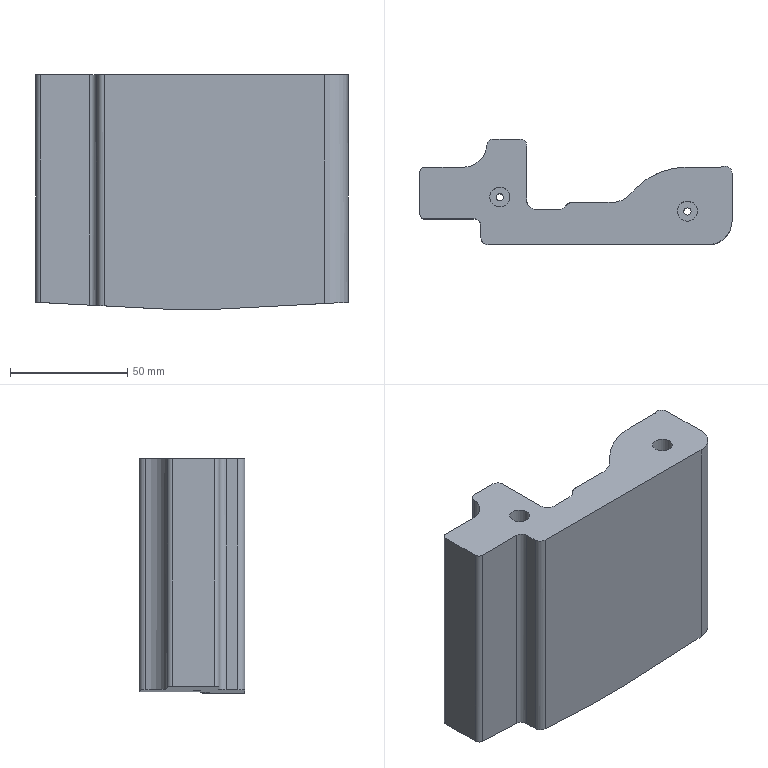Part | STEP file | lll_id234_x_t | 1 solid | 43 faces | box 133 x 45 x 100 mm | volume 339340 mm3 | cylinder 24 | plane 19 | commonest cylinder face diameters 6 x6 20 x3 3.1 x2 4 x2 8 x2 8.506 x2
STEP:
#1=CARTESIAN_POINT('',(1388.5,7.5,-7.5));
#2=VERTEX_POINT('',#1);
#3=CARTESIAN_POINT('',(1408.5,7.5,-7.5));
#4=VERTEX_POINT('',#3);
#5=CARTESIAN_POINT('',(1374.507,7.5,-7.5));
#6=DIRECTION('',(1.,0.,0.));
#7=VECTOR('',#6,1.);
#8=LINE('',#5,#7);
#9=EDGE_CURVE('',#2,#4,#8,.T.);
#10=ORIENTED_EDGE('',*,*,#9,.F.);
#11=CARTESIAN_POINT('',(1388.5,22.495,-7.5));
#12=VERTEX_POINT('',#11);
#13=CARTESIAN_POINT('',(1388.5,49.5,-7.5));
#14=DIRECTION('',(0.,-1.,0.));
#15=VECTOR('',#14,1.);
#16=LINE('',#13,#15);
#17=EDGE_CURVE('',#12,#2,#16,.T.);
#18=ORIENTED_EDGE('',*,*,#17,.F.);
#19=CARTESIAN_POINT('',(1391.,22.495,-7.5));
#20=VERTEX_POINT('',#19);
#21=CARTESIAN_POINT('',(1374.513,22.492,-7.5));
#22=DIRECTION('',(-1.,-0.0002273,0.));
#23=VECTOR('',#22,1.);
#24=LINE('',#21,#23);
#25=EDGE_CURVE('',#20,#12,#24,.T.);
#26=ORIENTED_EDGE('',*,*,#25,.F.);
#27=CARTESIAN_POINT('',(1394.112,23.983,-7.5));
#28=VERTEX_POINT('',#27);
#29=CARTESIAN_POINT('',(1390.999,26.495,-7.5));
#30=DIRECTION('',(0.,0.,-1.));
#31=DIRECTION('',(1.,0.,0.));
#32=AXIS2_PLACEMENT_3D('',#29,#30,#31);
#33=CIRCLE('',#32,4.);
#34=EDGE_CURVE('',#28,#20,#33,.T.);
#35=ORIENTED_EDGE('',*,*,#34,.F.);
#36=CARTESIAN_POINT('',(1394.775,24.627,-7.5));
#37=VERTEX_POINT('',#36);
#38=CARTESIAN_POINT('',(1397.092,21.579,-7.5));
#39=DIRECTION('',(0.,0.,1.));
#40=DIRECTION('',(1.,0.,0.));
#41=AXIS2_PLACEMENT_3D('',#38,#39,#40);
#42=CIRCLE('',#41,3.829);
#43=EDGE_CURVE('',#37,#28,#42,.T.);
#44=ORIENTED_EDGE('',*,*,#43,.F.);
#45=CARTESIAN_POINT('',(1395.716,25.182,-7.5));
#46=VERTEX_POINT('',#45);
#47=CARTESIAN_POINT('',(1397.363,21.312,-7.5));
#48=DIRECTION('',(0.,0.,1.));
#49=DIRECTION('',(1.,0.,0.));
#50=AXIS2_PLACEMENT_3D('',#47,#48,#49);
#51=CIRCLE('',#50,4.206);
#52=EDGE_CURVE('',#46,#37,#51,.T.);
#53=ORIENTED_EDGE('',*,*,#52,.F.);
#54=CARTESIAN_POINT('',(1396.385,25.384,-7.5));
#55=VERTEX_POINT('',#54);
#56=CARTESIAN_POINT('',(1397.014,22.085,-7.5));
#57=DIRECTION('',(0.,0.,1.));
#58=DIRECTION('',(1.,0.,0.));
#59=AXIS2_PLACEMENT_3D('',#56,#57,#58);
#60=CIRCLE('',#59,3.358);
#61=EDGE_CURVE('',#55,#46,#60,.T.);
#62=ORIENTED_EDGE('',*,*,#61,.F.);
#63=CARTESIAN_POINT('',(1396.692,25.434,-7.5));
#64=VERTEX_POINT('',#63);
#65=CARTESIAN_POINT('',(1397.334,20.531,-7.5));
#66=DIRECTION('',(0.,0.,-1.));
#67=DIRECTION('',(1.,0.,0.));
#68=AXIS2_PLACEMENT_3D('',#65,#66,#67);
#69=CIRCLE('',#68,4.944);
#70=EDGE_CURVE('',#55,#64,#69,.T.);
#71=ORIENTED_EDGE('',*,*,#70,.T.);
#72=CARTESIAN_POINT('',(1397.002,25.469,-7.5));
#73=VERTEX_POINT('',#72);
#74=CARTESIAN_POINT('',(1397.824,16.86,-7.5));
#75=DIRECTION('',(0.,0.,1.));
#76=DIRECTION('',(1.,0.,0.));
#77=AXIS2_PLACEMENT_3D('',#74,#75,#76);
#78=CIRCLE('',#77,8.648);
#79=EDGE_CURVE('',#73,#64,#78,.T.);
#80=ORIENTED_EDGE('',*,*,#79,.F.);
#81=CARTESIAN_POINT('',(1397.315,25.497,-7.5));
#82=VERTEX_POINT('',#81);
#83=CARTESIAN_POINT('',(1398.554,9.871,-7.5));
#84=DIRECTION('',(0.,0.,1.));
#85=DIRECTION('',(1.,0.,0.));
#86=AXIS2_PLACEMENT_3D('',#83,#84,#85);
#87=CIRCLE('',#86,15.675);
#88=EDGE_CURVE('',#82,#73,#87,.T.);
#89=ORIENTED_EDGE('',*,*,#88,.F.);
#90=CARTESIAN_POINT('',(1399.134,25.498,-7.5));
#91=VERTEX_POINT('',#90);
#92=CARTESIAN_POINT('',(1374.518,25.486,-7.5));
#93=DIRECTION('',(1.,0.0004734,0.));
#94=VECTOR('',#93,1.);
#95=LINE('',#92,#94);
#96=EDGE_CURVE('',#82,#91,#95,.T.);
#97=ORIENTED_EDGE('',*,*,#96,.T.);
#98=CARTESIAN_POINT('',(1408.5,25.502,-7.5));
#99=VERTEX_POINT('',#98);
#100=CARTESIAN_POINT('',(1374.517,25.488,-7.5));
#101=DIRECTION('',(1.,0.0004015,0.));
#102=VECTOR('',#101,1.);
#103=LINE('',#100,#102);
#104=EDGE_CURVE('',#91,#99,#103,.T.);
#105=ORIENTED_EDGE('',*,*,#104,.T.);
#106=CARTESIAN_POINT('',(1408.5,52.5,-7.5));
#107=DIRECTION('',(0.,1.,0.));
#108=VECTOR('',#107,1.);
#109=LINE('',#106,#108);
#110=EDGE_CURVE('',#4,#99,#109,.T.);
#111=ORIENTED_EDGE('',*,*,#110,.F.);
#112=EDGE_LOOP('',(#10,#18,#26,#35,#44,#53,#62,#71,#80,#89,#97,#105,#111));
#113=FACE_OUTER_BOUND('',#112,.T.);
#114=CARTESIAN_POINT('',(1374.507,49.5,-7.5));
#115=DIRECTION('',(0.,0.,1.));
#116=DIRECTION('',(-1.,0.,0.));
#117=AXIS2_PLACEMENT_3D('',#114,#115,#116);
#118=PLANE('',#117);
#119=ADVANCED_FACE('',(#113),#118,.F.);
#120=CARTESIAN_POINT('',(1370.253,27.75,92.5));
#121=VERTEX_POINT('',#120);
#122=CARTESIAN_POINT('',(1366.,27.75,92.5));
#123=DIRECTION('',(0.,0.,-1.));
#124=DIRECTION('',(1.,0.,0.));
#125=AXIS2_PLACEMENT_3D('',#122,#123,#124);
#126=CIRCLE('',#125,4.253);
#127=EDGE_CURVE('',#121,#121,#126,.T.);
#128=ORIENTED_EDGE('',*,*,#127,.T.);
#129=EDGE_LOOP('',(#128));
#130=FACE_BOUND('',#129,.T.);
#131=CARTESIAN_POINT('',(1450.253,21.75,92.5));
#132=VERTEX_POINT('',#131);
#133=CARTESIAN_POINT('',(1446.,21.75,92.5));
#134=DIRECTION('',(0.,0.,-1.));
#135=DIRECTION('',(1.,0.,0.));
#136=AXIS2_PLACEMENT_3D('',#133,#134,#135);
#137=CIRCLE('',#136,4.253);
#138=EDGE_CURVE('',#132,#132,#137,.T.);
#139=ORIENTED_EDGE('',*,*,#138,.T.);
#140=EDGE_LOOP('',(#139));
#141=FACE_BOUND('',#140,.T.);
#142=CARTESIAN_POINT('',(1394.775,24.627,92.5));
#143=VERTEX_POINT('',#142);
#144=CARTESIAN_POINT('',(1395.716,25.182,92.5));
#145=VERTEX_POINT('',#144);
#146=CARTESIAN_POINT('',(1397.363,21.312,92.5));
#147=DIRECTION('',(0.,0.,-1.));
#148=DIRECTION('',(1.,0.,0.));
#149=AXIS2_PLACEMENT_3D('',#146,#147,#148);
#150=CIRCLE('',#149,4.206);
#151=EDGE_CURVE('',#143,#145,#150,.T.);
#152=ORIENTED_EDGE('',*,*,#151,.F.);
#153=CARTESIAN_POINT('',(1394.112,23.983,92.5));
#154=VERTEX_POINT('',#153);
#155=CARTESIAN_POINT('',(1397.092,21.579,92.5));
#156=DIRECTION('',(0.,0.,1.));
#157=DIRECTION('',(1.,0.,0.));
#158=AXIS2_PLACEMENT_3D('',#155,#156,#157);
#159=CIRCLE('',#158,3.829);
#160=EDGE_CURVE('',#143,#154,#159,.T.);
#161=ORIENTED_EDGE('',*,*,#160,.T.);
#162=CARTESIAN_POINT('',(1391.,22.495,92.5));
#163=VERTEX_POINT('',#162);
#164=CARTESIAN_POINT('',(1390.999,26.495,92.5));
#165=DIRECTION('',(0.,0.,-1.));
#166=DIRECTION('',(1.,0.,0.));
#167=AXIS2_PLACEMENT_3D('',#164,#165,#166);
#168=CIRCLE('',#167,4.);
#169=EDGE_CURVE('',#154,#163,#168,.T.);
#170=ORIENTED_EDGE('',*,*,#169,.T.);
#171=CARTESIAN_POINT('',(1381.51,22.493,92.5));
#172=VERTEX_POINT('',#171);
#173=CARTESIAN_POINT('',(1374.513,22.492,92.5));
#174=DIRECTION('',(-1.,-0.0002273,0.));
#175=VECTOR('',#174,1.);
#176=LINE('',#173,#175);
#177=EDGE_CURVE('',#163,#172,#176,.T.);
#178=ORIENTED_EDGE('',*,*,#177,.T.);
#179=CARTESIAN_POINT('',(1377.509,26.493,92.5));
#180=VERTEX_POINT('',#179);
#181=CARTESIAN_POINT('',(1381.509,26.493,92.5));
#182=DIRECTION('',(0.,0.,1.));
#183=DIRECTION('',(1.,0.,0.));
#184=AXIS2_PLACEMENT_3D('',#181,#182,#183);
#185=CIRCLE('',#184,4.);
#186=EDGE_CURVE('',#180,#172,#185,.T.);
#187=ORIENTED_EDGE('',*,*,#186,.F.);
#188=CARTESIAN_POINT('',(1377.507,49.5,92.5));
#189=VERTEX_POINT('',#188);
#190=CARTESIAN_POINT('',(1377.507,49.5,92.5));
#191=DIRECTION('',(0.00008306,-1.,0.));
#192=VECTOR('',#191,1.);
#193=LINE('',#190,#192);
#194=EDGE_CURVE('',#189,#180,#193,.T.);
#195=ORIENTED_EDGE('',*,*,#194,.F.);
#196=CARTESIAN_POINT('',(1374.507,52.5,92.5));
#197=VERTEX_POINT('',#196);
#198=CARTESIAN_POINT('',(1374.507,49.5,92.5));
#199=DIRECTION('',(0.,0.,1.));
#200=DIRECTION('',(1.,0.,0.));
#201=AXIS2_PLACEMENT_3D('',#198,#199,#200);
#202=CIRCLE('',#201,3.);
#203=EDGE_CURVE('',#189,#197,#202,.T.);
#204=ORIENTED_EDGE('',*,*,#203,.T.);
#205=CARTESIAN_POINT('',(1363.461,52.5,92.5));
#206=VERTEX_POINT('',#205);
#207=CARTESIAN_POINT('',(1374.507,52.5,92.5));
#208=DIRECTION('',(-1.,0.,0.));
#209=VECTOR('',#208,1.);
#210=LINE('',#207,#209);
#211=EDGE_CURVE('',#197,#206,#210,.T.);
#212=ORIENTED_EDGE('',*,*,#211,.T.);
#213=CARTESIAN_POINT('',(1360.47,49.731,92.5));
#214=VERTEX_POINT('',#213);
#215=CARTESIAN_POINT('',(1363.461,49.5,92.5));
#216=DIRECTION('',(0.,0.,-1.));
#217=DIRECTION('',(1.,0.,0.));
#218=AXIS2_PLACEMENT_3D('',#215,#216,#217);
#219=CIRCLE('',#218,3.);
#220=EDGE_CURVE('',#214,#206,#219,.T.);
#221=ORIENTED_EDGE('',*,*,#220,.F.);
#222=CARTESIAN_POINT('',(1350.5,40.5,92.5));
#223=VERTEX_POINT('',#222);
#224=CARTESIAN_POINT('',(1350.5,50.5,92.5));
#225=DIRECTION('',(0.,0.,1.));
#226=DIRECTION('',(1.,0.,0.));
#227=AXIS2_PLACEMENT_3D('',#224,#225,#226);
#228=CIRCLE('',#227,10.);
#229=EDGE_CURVE('',#223,#214,#228,.T.);
#230=ORIENTED_EDGE('',*,*,#229,.F.);
#231=CARTESIAN_POINT('',(1334.,40.5,92.5));
#232=VERTEX_POINT('',#231);
#233=CARTESIAN_POINT('',(1374.507,40.5,92.5));
#234=DIRECTION('',(1.,0.,0.));
#235=VECTOR('',#234,1.);
#236=LINE('',#233,#235);
#237=EDGE_CURVE('',#232,#223,#236,.T.);
#238=ORIENTED_EDGE('',*,*,#237,.F.);
#239=CARTESIAN_POINT('',(1332.,38.5,92.5));
#240=VERTEX_POINT('',#239);
#241=CARTESIAN_POINT('',(1334.,38.5,92.5));
#242=DIRECTION('',(0.,0.,1.));
#243=DIRECTION('',(1.,0.,0.));
#244=AXIS2_PLACEMENT_3D('',#241,#242,#243);
#245=CIRCLE('',#244,2.);
#246=EDGE_CURVE('',#232,#240,#245,.T.);
#247=ORIENTED_EDGE('',*,*,#246,.T.);
#248=CARTESIAN_POINT('',(1332.,20.5,92.5));
#249=VERTEX_POINT('',#248);
#250=CARTESIAN_POINT('',(1332.,49.5,92.5));
#251=DIRECTION('',(0.,1.,0.));
#252=VECTOR('',#251,1.);
#253=LINE('',#250,#252);
#254=EDGE_CURVE('',#249,#240,#253,.T.);
#255=ORIENTED_EDGE('',*,*,#254,.F.);
#256=CARTESIAN_POINT('',(1334.,18.5,92.5));
#257=VERTEX_POINT('',#256);
#258=CARTESIAN_POINT('',(1334.,20.5,92.5));
#259=DIRECTION('',(0.,0.,1.));
#260=DIRECTION('',(1.,0.,0.));
#261=AXIS2_PLACEMENT_3D('',#258,#259,#260);
#262=CIRCLE('',#261,2.);
#263=EDGE_CURVE('',#249,#257,#262,.T.);
#264=ORIENTED_EDGE('',*,*,#263,.T.);
#265=CARTESIAN_POINT('',(1355.,18.5,92.5));
#266=VERTEX_POINT('',#265);
#267=CARTESIAN_POINT('',(1374.507,18.5,92.5));
#268=DIRECTION('',(1.,0.,0.));
#269=VECTOR('',#268,1.);
#270=LINE('',#267,#269);
#271=EDGE_CURVE('',#257,#266,#270,.T.);
#272=ORIENTED_EDGE('',*,*,#271,.T.);
#273=CARTESIAN_POINT('',(1358.,15.5,92.5));
#274=VERTEX_POINT('',#273);
#275=CARTESIAN_POINT('',(1355.,15.5,92.5));
#276=DIRECTION('',(0.,0.,1.));
#277=DIRECTION('',(1.,0.,0.));
#278=AXIS2_PLACEMENT_3D('',#275,#276,#277);
#279=CIRCLE('',#278,3.);
#280=EDGE_CURVE('',#274,#266,#279,.T.);
#281=ORIENTED_EDGE('',*,*,#280,.F.);
#282=CARTESIAN_POINT('',(1358.,10.5,92.5));
#283=VERTEX_POINT('',#282);
#284=CARTESIAN_POINT('',(1358.,49.5,92.5));
#285=DIRECTION('',(0.,1.,0.));
#286=VECTOR('',#285,1.);
#287=LINE('',#284,#286);
#288=EDGE_CURVE('',#283,#274,#287,.T.);
#289=ORIENTED_EDGE('',*,*,#288,.F.);
#290=CARTESIAN_POINT('',(1361.,7.5,92.5));
#291=VERTEX_POINT('',#290);
#292=CARTESIAN_POINT('',(1361.,10.5,92.5));
#293=DIRECTION('',(0.,0.,-1.));
#294=DIRECTION('',(1.,0.,0.));
#295=AXIS2_PLACEMENT_3D('',#292,#293,#294);
#296=CIRCLE('',#295,3.);
#297=EDGE_CURVE('',#291,#283,#296,.T.);
#298=ORIENTED_EDGE('',*,*,#297,.F.);
#299=CARTESIAN_POINT('',(1455.,7.5,92.5));
#300=VERTEX_POINT('',#299);
#301=CARTESIAN_POINT('',(1374.507,7.5,92.5));
#302=DIRECTION('',(1.,0.,0.));
#303=VECTOR('',#302,1.);
#304=LINE('',#301,#303);
#305=EDGE_CURVE('',#291,#300,#304,.T.);
#306=ORIENTED_EDGE('',*,*,#305,.T.);
#307=CARTESIAN_POINT('',(1465.,17.5,92.5));
#308=VERTEX_POINT('',#307);
#309=CARTESIAN_POINT('',(1455.,17.5,92.5));
#310=DIRECTION('',(0.,0.,-1.));
#311=DIRECTION('',(1.,0.,0.));
#312=AXIS2_PLACEMENT_3D('',#309,#310,#311);
#313=CIRCLE('',#312,10.);
#314=EDGE_CURVE('',#308,#300,#313,.T.);
#315=ORIENTED_EDGE('',*,*,#314,.F.);
#316=CARTESIAN_POINT('',(1465.,38.,92.5));
#317=VERTEX_POINT('',#316);
#318=CARTESIAN_POINT('',(1465.,49.5,92.5));
#319=DIRECTION('',(0.,1.,0.));
#320=VECTOR('',#319,1.);
#321=LINE('',#318,#320);
#322=EDGE_CURVE('',#308,#317,#321,.T.);
#323=ORIENTED_EDGE('',*,*,#322,.T.);
#324=CARTESIAN_POINT('',(1460.801,40.75,92.5));
#325=VERTEX_POINT('',#324);
#326=CARTESIAN_POINT('',(1462.,38.,92.5));
#327=DIRECTION('',(0.,0.,1.));
#328=DIRECTION('',(1.,0.,0.));
#329=AXIS2_PLACEMENT_3D('',#326,#327,#328);
#330=CIRCLE('',#329,3.);
#331=EDGE_CURVE('',#317,#325,#330,.T.);
#332=ORIENTED_EDGE('',*,*,#331,.T.);
#333=CARTESIAN_POINT('',(1459.602,40.5,92.5));
#334=VERTEX_POINT('',#333);
#335=CARTESIAN_POINT('',(1459.602,43.5,92.5));
#336=DIRECTION('',(0.,0.,-1.));
#337=DIRECTION('',(1.,0.,0.));
#338=AXIS2_PLACEMENT_3D('',#335,#336,#337);
#339=CIRCLE('',#338,3.);
#340=EDGE_CURVE('',#325,#334,#339,.T.);
#341=ORIENTED_EDGE('',*,*,#340,.T.);
#342=CARTESIAN_POINT('',(1445.426,40.5,92.5));
#343=VERTEX_POINT('',#342);
#344=CARTESIAN_POINT('',(1374.507,40.5,92.5));
#345=DIRECTION('',(1.,0.,0.));
#346=VECTOR('',#345,1.);
#347=LINE('',#344,#346);
#348=EDGE_CURVE('',#343,#334,#347,.T.);
#349=ORIENTED_EDGE('',*,*,#348,.F.);
#350=CARTESIAN_POINT('',(1424.213,31.713,92.5));
#351=VERTEX_POINT('',#350);
#352=CARTESIAN_POINT('',(1445.426,10.502,92.5));
#353=DIRECTION('',(0.,0.,-1.));
#354=DIRECTION('',(1.,0.,0.));
#355=AXIS2_PLACEMENT_3D('',#352,#353,#354);
#356=CIRCLE('',#355,29.998);
#357=EDGE_CURVE('',#351,#343,#356,.T.);
#358=ORIENTED_EDGE('',*,*,#357,.F.);
#359=CARTESIAN_POINT('',(1420.933,28.433,92.5));
#360=VERTEX_POINT('',#359);
#361=CARTESIAN_POINT('',(1408.253,15.754,92.5));
#362=DIRECTION('',(-0.7071,-0.7071,0.));
#363=VECTOR('',#362,1.);
#364=LINE('',#361,#363);
#365=EDGE_CURVE('',#351,#360,#364,.T.);
#366=ORIENTED_EDGE('',*,*,#365,.T.);
#367=CARTESIAN_POINT('',(1413.865,25.504,92.5));
#368=VERTEX_POINT('',#367);
#369=CARTESIAN_POINT('',(1413.861,35.504,92.5));
#370=DIRECTION('',(0.,0.,-1.));
#371=DIRECTION('',(1.,0.,0.));
#372=AXIS2_PLACEMENT_3D('',#369,#370,#371);
#373=CIRCLE('',#372,10.);
#374=EDGE_CURVE('',#360,#368,#373,.T.);
#375=ORIENTED_EDGE('',*,*,#374,.T.);
#376=CARTESIAN_POINT('',(1399.134,25.498,92.5));
#377=VERTEX_POINT('',#376);
#378=CARTESIAN_POINT('',(1374.517,25.488,92.5));
#379=DIRECTION('',(-1.,-0.0004015,0.));
#380=VECTOR('',#379,1.);
#381=LINE('',#378,#380);
#382=EDGE_CURVE('',#368,#377,#381,.T.);
#383=ORIENTED_EDGE('',*,*,#382,.T.);
#384=CARTESIAN_POINT('',(1397.315,25.497,92.5));
#385=VERTEX_POINT('',#384);
#386=CARTESIAN_POINT('',(1374.518,25.486,92.5));
#387=DIRECTION('',(1.,0.0004734,0.));
#388=VECTOR('',#387,1.);
#389=LINE('',#386,#388);
#390=EDGE_CURVE('',#385,#377,#389,.T.);
#391=ORIENTED_EDGE('',*,*,#390,.F.);
#392=CARTESIAN_POINT('',(1397.002,25.469,92.5));
#393=VERTEX_POINT('',#392);
#394=CARTESIAN_POINT('',(1398.554,9.871,92.5));
#395=DIRECTION('',(0.,0.,1.));
#396=DIRECTION('',(1.,0.,0.));
#397=AXIS2_PLACEMENT_3D('',#394,#395,#396);
#398=CIRCLE('',#397,15.675);
#399=EDGE_CURVE('',#385,#393,#398,.T.);
#400=ORIENTED_EDGE('',*,*,#399,.T.);
#401=CARTESIAN_POINT('',(1396.692,25.434,92.5));
#402=VERTEX_POINT('',#401);
#403=CARTESIAN_POINT('',(1397.824,16.86,92.5));
#404=DIRECTION('',(0.,0.,-1.));
#405=DIRECTION('',(1.,0.,0.));
#406=AXIS2_PLACEMENT_3D('',#403,#404,#405);
#407=CIRCLE('',#406,8.648);
#408=EDGE_CURVE('',#402,#393,#407,.T.);
#409=ORIENTED_EDGE('',*,*,#408,.F.);
#410=CARTESIAN_POINT('',(1396.385,25.384,92.5));
#411=VERTEX_POINT('',#410);
#412=CARTESIAN_POINT('',(1397.334,20.531,92.5));
#413=DIRECTION('',(0.,0.,1.));
#414=DIRECTION('',(1.,0.,0.));
#415=AXIS2_PLACEMENT_3D('',#412,#413,#414);
#416=CIRCLE('',#415,4.944);
#417=EDGE_CURVE('',#402,#411,#416,.T.);
#418=ORIENTED_EDGE('',*,*,#417,.T.);
#419=CARTESIAN_POINT('',(1397.014,22.085,92.5));
#420=DIRECTION('',(0.,0.,-1.));
#421=DIRECTION('',(1.,0.,0.));
#422=AXIS2_PLACEMENT_3D('',#419,#420,#421);
#423=CIRCLE('',#422,3.358);
#424=EDGE_CURVE('',#145,#411,#423,.T.);
#425=ORIENTED_EDGE('',*,*,#424,.F.);
#426=EDGE_LOOP('',(#152,#161,#170,#178,#187,#195,#204,#212,#221,#230,#238,#247,#255,#264,#272,#281,#289,#298,#306,#315,#323,#332,#341,#349,#358,#366,#375,#383,#391,#400,#409,#418,#425));
#427=FACE_BOUND('',#426,.T.);
#428=CARTESIAN_POINT('',(1374.507,49.5,92.5));
#429=DIRECTION('',(0.,0.,1.));
#430=DIRECTION('',(-1.,0.,0.));
#431=AXIS2_PLACEMENT_3D('',#428,#429,#430);
#432=PLANE('',#431);
#433=ADVANCED_FACE('',(#130,#141,#427),#432,.T.);
#434=CARTESIAN_POINT('',(1444.45,21.75,-5.591));
#435=VERTEX_POINT('',#434);
#436=CARTESIAN_POINT('',(1446.,21.75,-5.509));
#437=DIRECTION('',(-0.05302,0.,0.9986));
#438=DIRECTION('',(-0.9986,0.,-0.05302));
#439=AXIS2_PLACEMENT_3D('',#436,#437,#438);
#440=ELLIPSE('',#439,1.552,1.55);
#441=EDGE_CURVE('',#435,#435,#440,.T.);
#442=ORIENTED_EDGE('',*,*,#441,.T.);
#443=EDGE_LOOP('',(#442));
#444=FACE_BOUND('',#443,.T.);
#445=CARTESIAN_POINT('',(1455.,7.5,-5.031));
#446=VERTEX_POINT('',#445);
#447=CARTESIAN_POINT('',(1465.,17.5,-4.5));
#448=VERTEX_POINT('',#447);
#449=CARTESIAN_POINT('',(1455.,17.5,-5.031));
#450=DIRECTION('',(-0.05302,0.,0.9986));
#451=DIRECTION('',(0.9986,0.,0.05302));
#452=AXIS2_PLACEMENT_3D('',#449,#450,#451);
#453=ELLIPSE('',#452,10.014,10.);
#454=EDGE_CURVE('',#446,#448,#453,.T.);
#455=ORIENTED_EDGE('',*,*,#454,.F.);
#456=CARTESIAN_POINT('',(1408.5,7.5,-7.5));
#457=DIRECTION('',(0.9986,0.,0.05302));
#458=VECTOR('',#457,1.);
#459=LINE('',#456,#458);
#460=EDGE_CURVE('',#4,#446,#459,.T.);
#461=ORIENTED_EDGE('',*,*,#460,.F.);
#462=ORIENTED_EDGE('',*,*,#110,.T.);
#463=CARTESIAN_POINT('',(1413.865,25.504,-7.215));
#464=VERTEX_POINT('',#463);
#465=CARTESIAN_POINT('',(1408.511,25.502,-7.499));
#466=DIRECTION('',(0.9986,0.0004009,0.05302));
#467=VECTOR('',#466,1.);
#468=LINE('',#465,#467);
#469=EDGE_CURVE('',#99,#464,#468,.T.);
#470=ORIENTED_EDGE('',*,*,#469,.T.);
#471=CARTESIAN_POINT('',(1420.933,28.433,-6.84));
#472=VERTEX_POINT('',#471);
#473=CARTESIAN_POINT('',(1413.861,35.504,-7.215));
#474=DIRECTION('',(0.05302,0.,-0.9986));
#475=DIRECTION('',(0.9986,0.,0.05302));
#476=AXIS2_PLACEMENT_3D('',#473,#474,#475);
#477=ELLIPSE('',#476,10.014,10.);
#478=EDGE_CURVE('',#472,#464,#477,.T.);
#479=ORIENTED_EDGE('',*,*,#478,.F.);
#480=CARTESIAN_POINT('',(1424.213,31.713,-6.666));
#481=VERTEX_POINT('',#480);
#482=CARTESIAN_POINT('',(1426.724,34.224,-6.532));
#483=DIRECTION('',(0.7066,0.7066,0.03752));
#484=VECTOR('',#483,1.);
#485=LINE('',#482,#484);
#486=EDGE_CURVE('',#472,#481,#485,.T.);
#487=ORIENTED_EDGE('',*,*,#486,.T.);
#488=CARTESIAN_POINT('',(1445.426,40.5,-5.539));
#489=VERTEX_POINT('',#488);
#490=CARTESIAN_POINT('',(1445.426,10.502,-5.539));
#491=DIRECTION('',(-0.05302,0.,0.9986));
#492=DIRECTION('',(0.9986,0.,0.05302));
#493=AXIS2_PLACEMENT_3D('',#490,#491,#492);
#494=ELLIPSE('',#493,30.04,29.998);
#495=EDGE_CURVE('',#489,#481,#494,.T.);
#496=ORIENTED_EDGE('',*,*,#495,.F.);
#497=CARTESIAN_POINT('',(1459.602,40.5,-4.787));
#498=VERTEX_POINT('',#497);
#499=CARTESIAN_POINT('',(1408.5,40.5,-7.5));
#500=DIRECTION('',(0.9986,0.,0.05302));
#501=VECTOR('',#500,1.);
#502=LINE('',#499,#501);
#503=EDGE_CURVE('',#489,#498,#502,.T.);
#504=ORIENTED_EDGE('',*,*,#503,.T.);
#505=CARTESIAN_POINT('',(1460.801,40.75,-4.723));
#506=VERTEX_POINT('',#505);
#507=CARTESIAN_POINT('',(1459.602,43.5,-4.787));
#508=DIRECTION('',(-0.05302,0.,0.9986));
#509=DIRECTION('',(0.9986,0.,0.05302));
#510=AXIS2_PLACEMENT_3D('',#507,#508,#509);
#511=ELLIPSE('',#510,3.004,3.);
#512=EDGE_CURVE('',#498,#506,#511,.T.);
#513=ORIENTED_EDGE('',*,*,#512,.T.);
#514=CARTESIAN_POINT('',(1465.,38.,-4.5));
#515=VERTEX_POINT('',#514);
#516=CARTESIAN_POINT('',(1462.,38.,-4.659));
#517=DIRECTION('',(0.05302,0.,-0.9986));
#518=DIRECTION('',(0.9986,0.,0.05302));
#519=AXIS2_PLACEMENT_3D('',#516,#517,#518);
#520=ELLIPSE('',#519,3.004,3.);
#521=EDGE_CURVE('',#506,#515,#520,.T.);
#522=ORIENTED_EDGE('',*,*,#521,.T.);
#523=CARTESIAN_POINT('',(1465.,52.5,-4.5));
#524=DIRECTION('',(0.,-1.,0.));
#525=VECTOR('',#524,1.);
#526=LINE('',#523,#525);
#527=EDGE_CURVE('',#515,#448,#526,.T.);
#528=ORIENTED_EDGE('',*,*,#527,.T.);
#529=EDGE_LOOP('',(#455,#461,#462,#470,#479,#487,#496,#504,#513,#522,#528));
#530=FACE_BOUND('',#529,.T.);
#531=CARTESIAN_POINT('',(1408.5,52.5,-7.5));
#532=DIRECTION('',(0.05302,0.,-0.9986));
#533=DIRECTION('',(-0.9986,0.,-0.05302));
#534=AXIS2_PLACEMENT_3D('',#531,#532,#533);
#535=PLANE('',#534);
#536=ADVANCED_FACE('',(#444,#530),#535,.T.);
#537=CARTESIAN_POINT('',(1367.55,27.75,-6.388));
#538=VERTEX_POINT('',#537);
#539=CARTESIAN_POINT('',(1366.,27.75,-6.305));
#540=DIRECTION('',(-0.05302,0.,-0.9986));
#541=DIRECTION('',(0.9986,0.,-0.05302));
#542=AXIS2_PLACEMENT_3D('',#539,#540,#541);
#543=ELLIPSE('',#542,1.552,1.55);
#544=EDGE_CURVE('',#538,#538,#543,.T.);
#545=ORIENTED_EDGE('',*,*,#544,.F.);
#546=EDGE_LOOP('',(#545));
#547=FACE_BOUND('',#546,.T.);
#548=CARTESIAN_POINT('',(1381.51,22.493,-7.129));
#549=VERTEX_POINT('',#548);
#550=CARTESIAN_POINT('',(1388.507,22.495,-7.5));
#551=DIRECTION('',(-0.9986,-0.000227,0.05302));
#552=VECTOR('',#551,1.);
#553=LINE('',#550,#552);
#554=EDGE_CURVE('',#12,#549,#553,.T.);
#555=ORIENTED_EDGE('',*,*,#554,.F.);
#556=ORIENTED_EDGE('',*,*,#17,.T.);
#557=CARTESIAN_POINT('',(1361.,7.5,-6.04));
#558=VERTEX_POINT('',#557);
#559=CARTESIAN_POINT('',(1388.5,7.5,-7.5));
#560=DIRECTION('',(-0.9986,0.,0.05302));
#561=VECTOR('',#560,1.);
#562=LINE('',#559,#561);
#563=EDGE_CURVE('',#2,#558,#562,.T.);
#564=ORIENTED_EDGE('',*,*,#563,.T.);
#565=CARTESIAN_POINT('',(1358.,10.5,-5.881));
#566=VERTEX_POINT('',#565);
#567=CARTESIAN_POINT('',(1361.,10.5,-6.04));
#568=DIRECTION('',(0.05302,0.,0.9986));
#569=DIRECTION('',(-0.9986,0.,0.05302));
#570=AXIS2_PLACEMENT_3D('',#567,#568,#569);
#571=ELLIPSE('',#570,3.004,3.);
#572=EDGE_CURVE('',#566,#558,#571,.T.);
#573=ORIENTED_EDGE('',*,*,#572,.F.);
#574=CARTESIAN_POINT('',(1358.,15.5,-5.881));
#575=VERTEX_POINT('',#574);
#576=CARTESIAN_POINT('',(1358.,52.5,-5.881));
#577=DIRECTION('',(0.,-1.,0.));
#578=VECTOR('',#577,1.);
#579=LINE('',#576,#578);
#580=EDGE_CURVE('',#575,#566,#579,.T.);
#581=ORIENTED_EDGE('',*,*,#580,.F.);
#582=CARTESIAN_POINT('',(1355.,18.5,-5.721));
#583=VERTEX_POINT('',#582);
#584=CARTESIAN_POINT('',(1355.,15.5,-5.721));
#585=DIRECTION('',(-0.05302,0.,-0.9986));
#586=DIRECTION('',(-0.9986,0.,0.05302));
#587=AXIS2_PLACEMENT_3D('',#584,#585,#586);
#588=ELLIPSE('',#587,3.004,3.);
#589=EDGE_CURVE('',#583,#575,#588,.T.);
#590=ORIENTED_EDGE('',*,*,#589,.F.);
#591=CARTESIAN_POINT('',(1334.,18.5,-4.606));
#592=VERTEX_POINT('',#591);
#593=CARTESIAN_POINT('',(1388.5,18.5,-7.5));
#594=DIRECTION('',(0.9986,0.,-0.05302));
#595=VECTOR('',#594,1.);
#596=LINE('',#593,#595);
#597=EDGE_CURVE('',#592,#583,#596,.T.);
#598=ORIENTED_EDGE('',*,*,#597,.F.);
#599=CARTESIAN_POINT('',(1332.,20.5,-4.5));
#600=VERTEX_POINT('',#599);
#601=CARTESIAN_POINT('',(1334.,20.5,-4.606));
#602=DIRECTION('',(0.05302,0.,0.9986));
#603=DIRECTION('',(-0.9986,0.,0.05302));
#604=AXIS2_PLACEMENT_3D('',#601,#602,#603);
#605=ELLIPSE('',#604,2.003,2.);
#606=EDGE_CURVE('',#600,#592,#605,.T.);
#607=ORIENTED_EDGE('',*,*,#606,.F.);
#608=CARTESIAN_POINT('',(1332.,38.5,-4.5));
#609=VERTEX_POINT('',#608);
#610=CARTESIAN_POINT('',(1332.,52.5,-4.5));
#611=DIRECTION('',(0.,1.,0.));
#612=VECTOR('',#611,1.);
#613=LINE('',#610,#612);
#614=EDGE_CURVE('',#600,#609,#613,.T.);
#615=ORIENTED_EDGE('',*,*,#614,.T.);
#616=CARTESIAN_POINT('',(1334.,40.5,-4.606));
#617=VERTEX_POINT('',#616);
#618=CARTESIAN_POINT('',(1334.,38.5,-4.606));
#619=DIRECTION('',(0.05302,0.,0.9986));
#620=DIRECTION('',(-0.9986,0.,0.05302));
#621=AXIS2_PLACEMENT_3D('',#618,#619,#620);
#622=ELLIPSE('',#621,2.003,2.);
#623=EDGE_CURVE('',#617,#609,#622,.T.);
#624=ORIENTED_EDGE('',*,*,#623,.F.);
#625=CARTESIAN_POINT('',(1350.5,40.5,-5.482));
#626=VERTEX_POINT('',#625);
#627=CARTESIAN_POINT('',(1388.5,40.5,-7.5));
#628=DIRECTION('',(-0.9986,0.,0.05302));
#629=VECTOR('',#628,1.);
#630=LINE('',#627,#629);
#631=EDGE_CURVE('',#626,#617,#630,.T.);
#632=ORIENTED_EDGE('',*,*,#631,.F.);
#633=CARTESIAN_POINT('',(1360.47,49.731,-6.012));
#634=VERTEX_POINT('',#633);
#635=CARTESIAN_POINT('',(1350.5,50.5,-5.482));
#636=DIRECTION('',(-0.05302,0.,-0.9986));
#637=DIRECTION('',(-0.9986,0.,0.05302));
#638=AXIS2_PLACEMENT_3D('',#635,#636,#637);
#639=ELLIPSE('',#638,10.014,10.);
#640=EDGE_CURVE('',#634,#626,#639,.T.);
#641=ORIENTED_EDGE('',*,*,#640,.F.);
#642=CARTESIAN_POINT('',(1363.461,52.5,-6.171));
#643=VERTEX_POINT('',#642);
#644=CARTESIAN_POINT('',(1363.461,49.5,-6.171));
#645=DIRECTION('',(0.05302,0.,0.9986));
#646=DIRECTION('',(-0.9986,0.,0.05302));
#647=AXIS2_PLACEMENT_3D('',#644,#645,#646);
#648=ELLIPSE('',#647,3.004,3.);
#649=EDGE_CURVE('',#643,#634,#648,.T.);
#650=ORIENTED_EDGE('',*,*,#649,.F.);
#651=CARTESIAN_POINT('',(1374.507,52.5,-6.757));
#652=VERTEX_POINT('',#651);
#653=CARTESIAN_POINT('',(1388.5,52.5,-7.5));
#654=DIRECTION('',(-0.9986,0.,0.05302));
#655=VECTOR('',#654,1.);
#656=LINE('',#653,#655);
#657=EDGE_CURVE('',#652,#643,#656,.T.);
#658=ORIENTED_EDGE('',*,*,#657,.F.);
#659=CARTESIAN_POINT('',(1377.507,49.5,-6.916));
#660=VERTEX_POINT('',#659);
#661=CARTESIAN_POINT('',(1374.507,49.5,-6.757));
#662=DIRECTION('',(0.05302,0.,0.9986));
#663=DIRECTION('',(-0.9986,0.,0.05302));
#664=AXIS2_PLACEMENT_3D('',#661,#662,#663);
#665=ELLIPSE('',#664,3.004,3.);
#666=EDGE_CURVE('',#660,#652,#665,.T.);
#667=ORIENTED_EDGE('',*,*,#666,.F.);
#668=CARTESIAN_POINT('',(1377.509,26.493,-6.916));
#669=VERTEX_POINT('',#668);
#670=CARTESIAN_POINT('',(1377.507,52.499,-6.916));
#671=DIRECTION('',(0.00008306,-1.,-0.00000441));
#672=VECTOR('',#671,1.);
#673=LINE('',#670,#672);
#674=EDGE_CURVE('',#660,#669,#673,.T.);
#675=ORIENTED_EDGE('',*,*,#674,.T.);
#676=CARTESIAN_POINT('',(1381.509,26.493,-7.129));
#677=DIRECTION('',(0.05302,0.,0.9986));
#678=DIRECTION('',(-0.9986,0.,0.05302));
#679=AXIS2_PLACEMENT_3D('',#676,#677,#678);
#680=ELLIPSE('',#679,4.006,4.);
#681=EDGE_CURVE('',#669,#549,#680,.T.);
#682=ORIENTED_EDGE('',*,*,#681,.T.);
#683=EDGE_LOOP('',(#555,#556,#564,#573,#581,#590,#598,#607,#615,#624,#632,#641,#650,#658,#667,#675,#682));
#684=FACE_BOUND('',#683,.T.);
#685=CARTESIAN_POINT('',(1388.5,52.5,-7.5));
#686=DIRECTION('',(0.05302,0.,0.9986));
#687=DIRECTION('',(0.9986,0.,-0.05302));
#688=AXIS2_PLACEMENT_3D('',#685,#686,#687);
#689=PLANE('',#688);
#690=ADVANCED_FACE('',(#547,#684),#689,.F.);
#691=ORIENTED_EDGE('',*,*,#441,.F.);
#692=EDGE_LOOP('',(#691));
#693=FACE_BOUND('',#692,.T.);
#694=CARTESIAN_POINT('',(1447.55,21.75,30.747));
#695=VERTEX_POINT('',#694);
#696=CARTESIAN_POINT('',(1446.,21.75,30.747));
#697=DIRECTION('',(0.,0.,-1.));
#698=DIRECTION('',(1.,0.,0.));
#699=AXIS2_PLACEMENT_3D('',#696,#697,#698);
#700=CIRCLE('',#699,1.55);
#701=EDGE_CURVE('',#695,#695,#700,.T.);
#702=ORIENTED_EDGE('',*,*,#701,.F.);
#703=EDGE_LOOP('',(#702));
#704=FACE_BOUND('',#703,.T.);
#705=CARTESIAN_POINT('',(1446.,21.75,37.747));
#706=DIRECTION('',(0.,0.,-1.));
#707=DIRECTION('',(-1.,0.,0.));
#708=AXIS2_PLACEMENT_3D('',#705,#706,#707);
#709=CYLINDRICAL_SURFACE('',#708,1.55);
#710=ADVANCED_FACE('',(#693,#704),#709,.F.);
#711=ORIENTED_EDGE('',*,*,#138,.F.);
#712=EDGE_LOOP('',(#711));
#713=FACE_BOUND('',#712,.T.);
#714=CARTESIAN_POINT('',(1441.747,21.75,30.747));
#715=VERTEX_POINT('',#714);
#716=CARTESIAN_POINT('',(1446.,21.75,30.747));
#717=DIRECTION('',(0.,0.,1.));
#718=DIRECTION('',(-1.,0.,0.));
#719=AXIS2_PLACEMENT_3D('',#716,#717,#718);
#720=CIRCLE('',#719,4.253);
#721=EDGE_CURVE('',#715,#715,#720,.T.);
#722=ORIENTED_EDGE('',*,*,#721,.F.);
#723=EDGE_LOOP('',(#722));
#724=FACE_BOUND('',#723,.T.);
#725=CARTESIAN_POINT('',(1446.,21.75,94.5));
#726=DIRECTION('',(0.,0.,-1.));
#727=DIRECTION('',(1.,0.,0.));
#728=AXIS2_PLACEMENT_3D('',#725,#726,#727);
#729=CYLINDRICAL_SURFACE('',#728,4.253);
#730=ADVANCED_FACE('',(#713,#724),#729,.F.);
#731=ORIENTED_EDGE('',*,*,#127,.F.);
#732=EDGE_LOOP('',(#731));
#733=FACE_BOUND('',#732,.T.);
#734=CARTESIAN_POINT('',(1361.747,27.75,30.747));
#735=VERTEX_POINT('',#734);
#736=CARTESIAN_POINT('',(1366.,27.75,30.747));
#737=DIRECTION('',(0.,0.,-1.));
#738=DIRECTION('',(-1.,0.,0.));
#739=AXIS2_PLACEMENT_3D('',#736,#737,#738);
#740=CIRCLE('',#739,4.253);
#741=EDGE_CURVE('',#735,#735,#740,.T.);
#742=ORIENTED_EDGE('',*,*,#741,.T.);
#743=EDGE_LOOP('',(#742));
#744=FACE_BOUND('',#743,.T.);
#745=CARTESIAN_POINT('',(1366.,27.75,94.5));
#746=DIRECTION('',(0.,0.,-1.));
#747=DIRECTION('',(1.,0.,0.));
#748=AXIS2_PLACEMENT_3D('',#745,#746,#747);
#749=CYLINDRICAL_SURFACE('',#748,4.253);
#750=ADVANCED_FACE('',(#733,#744),#749,.F.);
#751=CARTESIAN_POINT('',(1364.45,27.75,30.747));
#752=VERTEX_POINT('',#751);
#753=CARTESIAN_POINT('',(1366.,27.75,30.747));
#754=DIRECTION('',(0.,0.,1.));
#755=DIRECTION('',(-1.,0.,0.));
#756=AXIS2_PLACEMENT_3D('',#753,#754,#755);
#757=CIRCLE('',#756,1.55);
#758=EDGE_CURVE('',#752,#752,#757,.T.);
#759=ORIENTED_EDGE('',*,*,#758,.T.);
#760=EDGE_LOOP('',(#759));
#761=FACE_BOUND('',#760,.T.);
#762=ORIENTED_EDGE('',*,*,#544,.T.);
#763=EDGE_LOOP('',(#762));
#764=FACE_BOUND('',#763,.T.);
#765=CARTESIAN_POINT('',(1366.,27.75,37.747));
#766=DIRECTION('',(0.,0.,-1.));
#767=DIRECTION('',(-1.,0.,0.));
#768=AXIS2_PLACEMENT_3D('',#765,#766,#767);
#769=CYLINDRICAL_SURFACE('',#768,1.55);
#770=ADVANCED_FACE('',(#761,#764),#769,.F.);
#771=ORIENTED_EDGE('',*,*,#721,.T.);
#772=EDGE_LOOP('',(#771));
#773=FACE_BOUND('',#772,.T.);
#774=ORIENTED_EDGE('',*,*,#701,.T.);
#775=EDGE_LOOP('',(#774));
#776=FACE_BOUND('',#775,.T.);
#777=CARTESIAN_POINT('',(1446.,21.75,30.747));
#778=DIRECTION('',(0.,0.,1.));
#779=DIRECTION('',(1.,0.,0.));
#780=AXIS2_PLACEMENT_3D('',#777,#778,#779);
#781=PLANE('',#780);
#782=ADVANCED_FACE('',(#773,#776),#781,.T.);
#783=ORIENTED_EDGE('',*,*,#741,.F.);
#784=EDGE_LOOP('',(#783));
#785=FACE_BOUND('',#784,.T.);
#786=ORIENTED_EDGE('',*,*,#758,.F.);
#787=EDGE_LOOP('',(#786));
#788=FACE_BOUND('',#787,.T.);
#789=CARTESIAN_POINT('',(1366.,27.75,30.747));
#790=DIRECTION('',(0.,0.,-1.));
#791=DIRECTION('',(-1.,0.,0.));
#792=AXIS2_PLACEMENT_3D('',#789,#790,#791);
#793=PLANE('',#792);
#794=ADVANCED_FACE('',(#785,#788),#793,.F.);
#795=CARTESIAN_POINT('',(1394.775,24.627,-177.5));
#796=DIRECTION('',(0.,0.,1.));
#797=VECTOR('',#796,1.);
#798=LINE('',#795,#797);
#799=EDGE_CURVE('',#37,#143,#798,.T.);
#800=ORIENTED_EDGE('',*,*,#799,.F.);
#801=ORIENTED_EDGE('',*,*,#43,.T.);
#802=CARTESIAN_POINT('',(1394.112,23.983,-177.5));
#803=DIRECTION('',(0.,0.,1.));
#804=VECTOR('',#803,1.);
#805=LINE('',#802,#804);
#806=EDGE_CURVE('',#28,#154,#805,.T.);
#807=ORIENTED_EDGE('',*,*,#806,.T.);
#808=ORIENTED_EDGE('',*,*,#160,.F.);
#809=EDGE_LOOP('',(#800,#801,#807,#808));
#810=FACE_OUTER_BOUND('',#809,.T.);
#811=CARTESIAN_POINT('',(1397.092,21.579,-177.5));
#812=DIRECTION('',(0.,0.,1.));
#813=DIRECTION('',(1.,0.,0.));
#814=AXIS2_PLACEMENT_3D('',#811,#812,#813);
#815=CYLINDRICAL_SURFACE('',#814,3.829);
#816=ADVANCED_FACE('',(#810),#815,.T.);
#817=ORIENTED_EDGE('',*,*,#806,.F.);
#818=ORIENTED_EDGE('',*,*,#34,.T.);
#819=CARTESIAN_POINT('',(1391.,22.495,-177.5));
#820=DIRECTION('',(0.,0.,1.));
#821=VECTOR('',#820,1.);
#822=LINE('',#819,#821);
#823=EDGE_CURVE('',#20,#163,#822,.T.);
#824=ORIENTED_EDGE('',*,*,#823,.T.);
#825=ORIENTED_EDGE('',*,*,#169,.F.);
#826=EDGE_LOOP('',(#817,#818,#824,#825));
#827=FACE_OUTER_BOUND('',#826,.T.);
#828=CARTESIAN_POINT('',(1390.999,26.495,-177.5));
#829=DIRECTION('',(0.,0.,1.));
#830=DIRECTION('',(1.,0.,0.));
#831=AXIS2_PLACEMENT_3D('',#828,#829,#830);
#832=CYLINDRICAL_SURFACE('',#831,4.);
#833=ADVANCED_FACE('',(#827),#832,.F.);
#834=CARTESIAN_POINT('',(1399.134,25.498,-177.5));
#835=DIRECTION('',(0.,0.,1.));
#836=VECTOR('',#835,1.);
#837=LINE('',#834,#836);
#838=EDGE_CURVE('',#91,#377,#837,.T.);
#839=ORIENTED_EDGE('',*,*,#838,.F.);
#840=ORIENTED_EDGE('',*,*,#96,.F.);
#841=CARTESIAN_POINT('',(1397.315,25.497,-177.5));
#842=DIRECTION('',(0.,0.,1.));
#843=VECTOR('',#842,1.);
#844=LINE('',#841,#843);
#845=EDGE_CURVE('',#82,#385,#844,.T.);
#846=ORIENTED_EDGE('',*,*,#845,.T.);
#847=ORIENTED_EDGE('',*,*,#390,.T.);
#848=EDGE_LOOP('',(#839,#840,#846,#847));
#849=FACE_OUTER_BOUND('',#848,.T.);
#850=CARTESIAN_POINT('',(1399.134,25.498,-177.5));
#851=DIRECTION('',(-0.0004734,1.,0.));
#852=DIRECTION('',(-1.,-0.0004734,0.));
#853=AXIS2_PLACEMENT_3D('',#850,#851,#852);
#854=PLANE('',#853);
#855=ADVANCED_FACE('',(#849),#854,.T.);
#856=ORIENTED_EDGE('',*,*,#845,.F.);
#857=ORIENTED_EDGE('',*,*,#88,.T.);
#858=CARTESIAN_POINT('',(1397.002,25.469,-177.5));
#859=DIRECTION('',(0.,0.,1.));
#860=VECTOR('',#859,1.);
#861=LINE('',#858,#860);
#862=EDGE_CURVE('',#73,#393,#861,.T.);
#863=ORIENTED_EDGE('',*,*,#862,.T.);
#864=ORIENTED_EDGE('',*,*,#399,.F.);
#865=EDGE_LOOP('',(#856,#857,#863,#864));
#866=FACE_OUTER_BOUND('',#865,.T.);
#867=CARTESIAN_POINT('',(1398.554,9.871,-177.5));
#868=DIRECTION('',(0.,0.,1.));
#869=DIRECTION('',(1.,0.,0.));
#870=AXIS2_PLACEMENT_3D('',#867,#868,#869);
#871=CYLINDRICAL_SURFACE('',#870,15.675);
#872=ADVANCED_FACE('',(#866),#871,.T.);
#873=ORIENTED_EDGE('',*,*,#862,.F.);
#874=ORIENTED_EDGE('',*,*,#79,.T.);
#875=CARTESIAN_POINT('',(1396.692,25.434,-177.5));
#876=DIRECTION('',(0.,0.,1.));
#877=VECTOR('',#876,1.);
#878=LINE('',#875,#877);
#879=EDGE_CURVE('',#64,#402,#878,.T.);
#880=ORIENTED_EDGE('',*,*,#879,.T.);
#881=ORIENTED_EDGE('',*,*,#408,.T.);
#882=EDGE_LOOP('',(#873,#874,#880,#881));
#883=FACE_OUTER_BOUND('',#882,.T.);
#884=CARTESIAN_POINT('',(1397.824,16.86,-177.5));
#885=DIRECTION('',(0.,0.,1.));
#886=DIRECTION('',(1.,0.,0.));
#887=AXIS2_PLACEMENT_3D('',#884,#885,#886);
#888=CYLINDRICAL_SURFACE('',#887,8.648);
#889=ADVANCED_FACE('',(#883),#888,.T.);
#890=ORIENTED_EDGE('',*,*,#879,.F.);
#891=ORIENTED_EDGE('',*,*,#70,.F.);
#892=CARTESIAN_POINT('',(1396.385,25.384,-177.5));
#893=DIRECTION('',(0.,0.,1.));
#894=VECTOR('',#893,1.);
#895=LINE('',#892,#894);
#896=EDGE_CURVE('',#55,#411,#895,.T.);
#897=ORIENTED_EDGE('',*,*,#896,.T.);
#898=ORIENTED_EDGE('',*,*,#417,.F.);
#899=EDGE_LOOP('',(#890,#891,#897,#898));
#900=FACE_OUTER_BOUND('',#899,.T.);
#901=CARTESIAN_POINT('',(1397.334,20.531,-177.5));
#902=DIRECTION('',(0.,0.,1.));
#903=DIRECTION('',(1.,0.,0.));
#904=AXIS2_PLACEMENT_3D('',#901,#902,#903);
#905=CYLINDRICAL_SURFACE('',#904,4.944);
#906=ADVANCED_FACE('',(#900),#905,.T.);
#907=ORIENTED_EDGE('',*,*,#896,.F.);
#908=ORIENTED_EDGE('',*,*,#61,.T.);
#909=CARTESIAN_POINT('',(1395.716,25.182,-177.5));
#910=DIRECTION('',(0.,0.,1.));
#911=VECTOR('',#910,1.);
#912=LINE('',#909,#911);
#913=EDGE_CURVE('',#46,#145,#912,.T.);
#914=ORIENTED_EDGE('',*,*,#913,.T.);
#915=ORIENTED_EDGE('',*,*,#424,.T.);
#916=EDGE_LOOP('',(#907,#908,#914,#915));
#917=FACE_OUTER_BOUND('',#916,.T.);
#918=CARTESIAN_POINT('',(1397.014,22.085,-177.5));
#919=DIRECTION('',(0.,0.,1.));
#920=DIRECTION('',(1.,0.,0.));
#921=AXIS2_PLACEMENT_3D('',#918,#919,#920);
#922=CYLINDRICAL_SURFACE('',#921,3.358);
#923=ADVANCED_FACE('',(#917),#922,.T.);
#924=ORIENTED_EDGE('',*,*,#913,.F.);
#925=ORIENTED_EDGE('',*,*,#52,.T.);
#926=ORIENTED_EDGE('',*,*,#799,.T.);
#927=ORIENTED_EDGE('',*,*,#151,.T.);
#928=EDGE_LOOP('',(#924,#925,#926,#927));
#929=FACE_OUTER_BOUND('',#928,.T.);
#930=CARTESIAN_POINT('',(1397.363,21.312,-177.5));
#931=DIRECTION('',(0.,0.,1.));
#932=DIRECTION('',(1.,0.,0.));
#933=AXIS2_PLACEMENT_3D('',#930,#931,#932);
#934=CYLINDRICAL_SURFACE('',#933,4.206);
#935=ADVANCED_FACE('',(#929),#934,.T.);
#936=ORIENTED_EDGE('',*,*,#382,.F.);
#937=CARTESIAN_POINT('',(1413.865,25.504,-177.5));
#938=DIRECTION('',(0.,0.,1.));
#939=VECTOR('',#938,1.);
#940=LINE('',#937,#939);
#941=EDGE_CURVE('',#464,#368,#940,.T.);
#942=ORIENTED_EDGE('',*,*,#941,.F.);
#943=ORIENTED_EDGE('',*,*,#469,.F.);
#944=ORIENTED_EDGE('',*,*,#104,.F.);
#945=ORIENTED_EDGE('',*,*,#838,.T.);
#946=EDGE_LOOP('',(#936,#942,#943,#944,#945));
#947=FACE_OUTER_BOUND('',#946,.T.);
#948=CARTESIAN_POINT('',(1413.865,25.504,-177.5));
#949=DIRECTION('',(-0.0004015,1.,0.));
#950=DIRECTION('',(-1.,-0.0004015,0.));
#951=AXIS2_PLACEMENT_3D('',#948,#949,#950);
#952=PLANE('',#951);
#953=ADVANCED_FACE('',(#947),#952,.T.);
#954=ORIENTED_EDGE('',*,*,#177,.F.);
#955=ORIENTED_EDGE('',*,*,#823,.F.);
#956=ORIENTED_EDGE('',*,*,#25,.T.);
#957=ORIENTED_EDGE('',*,*,#554,.T.);
#958=CARTESIAN_POINT('',(1381.51,22.493,-177.5));
#959=DIRECTION('',(0.,0.,1.));
#960=VECTOR('',#959,1.);
#961=LINE('',#958,#960);
#962=EDGE_CURVE('',#549,#172,#961,.T.);
#963=ORIENTED_EDGE('',*,*,#962,.T.);
#964=EDGE_LOOP('',(#954,#955,#956,#957,#963));
#965=FACE_OUTER_BOUND('',#964,.T.);
#966=CARTESIAN_POINT('',(1391.,22.495,-177.5));
#967=DIRECTION('',(-0.0002273,1.,0.));
#968=DIRECTION('',(-1.,-0.0002273,0.));
#969=AXIS2_PLACEMENT_3D('',#966,#967,#968);
#970=PLANE('',#969);
#971=ADVANCED_FACE('',(#965),#970,.T.);
#972=ORIENTED_EDGE('',*,*,#186,.T.);
#973=ORIENTED_EDGE('',*,*,#962,.F.);
#974=ORIENTED_EDGE('',*,*,#681,.F.);
#975=CARTESIAN_POINT('',(1377.509,26.493,-177.5));
#976=DIRECTION('',(0.,0.,1.));
#977=VECTOR('',#976,1.);
#978=LINE('',#975,#977);
#979=EDGE_CURVE('',#669,#180,#978,.T.);
#980=ORIENTED_EDGE('',*,*,#979,.T.);
#981=EDGE_LOOP('',(#972,#973,#974,#980));
#982=FACE_OUTER_BOUND('',#981,.T.);
#983=CARTESIAN_POINT('',(1381.509,26.493,-177.5));
#984=DIRECTION('',(0.,0.,1.));
#985=DIRECTION('',(1.,0.,0.));
#986=AXIS2_PLACEMENT_3D('',#983,#984,#985);
#987=CYLINDRICAL_SURFACE('',#986,4.);
#988=ADVANCED_FACE('',(#982),#987,.F.);
#989=ORIENTED_EDGE('',*,*,#194,.T.);
#990=ORIENTED_EDGE('',*,*,#979,.F.);
#991=ORIENTED_EDGE('',*,*,#674,.F.);
#992=CARTESIAN_POINT('',(1377.507,49.5,-177.5));
#993=DIRECTION('',(0.,0.,1.));
#994=VECTOR('',#993,1.);
#995=LINE('',#992,#994);
#996=EDGE_CURVE('',#660,#189,#995,.T.);
#997=ORIENTED_EDGE('',*,*,#996,.T.);
#998=EDGE_LOOP('',(#989,#990,#991,#997));
#999=FACE_OUTER_BOUND('',#998,.T.);
#1000=CARTESIAN_POINT('',(1377.509,26.493,-177.5));
#1001=DIRECTION('',(1.,0.00008306,0.));
#1002=DIRECTION('',(-0.00008306,1.,0.));
#1003=AXIS2_PLACEMENT_3D('',#1000,#1001,#1002);
#1004=PLANE('',#1003);
#1005=ADVANCED_FACE('',(#999),#1004,.T.);
#1006=ORIENTED_EDGE('',*,*,#203,.F.);
#1007=ORIENTED_EDGE('',*,*,#996,.F.);
#1008=ORIENTED_EDGE('',*,*,#666,.T.);
#1009=CARTESIAN_POINT('',(1374.507,52.5,-177.5));
#1010=DIRECTION('',(0.,0.,1.));
#1011=VECTOR('',#1010,1.);
#1012=LINE('',#1009,#1011);
#1013=EDGE_CURVE('',#652,#197,#1012,.T.);
#1014=ORIENTED_EDGE('',*,*,#1013,.T.);
#1015=EDGE_LOOP('',(#1006,#1007,#1008,#1014));
#1016=FACE_OUTER_BOUND('',#1015,.T.);
#1017=CARTESIAN_POINT('',(1374.507,49.5,-177.5));
#1018=DIRECTION('',(0.,0.,1.));
#1019=DIRECTION('',(1.,0.,0.));
#1020=AXIS2_PLACEMENT_3D('',#1017,#1018,#1019);
#1021=CYLINDRICAL_SURFACE('',#1020,3.);
#1022=ADVANCED_FACE('',(#1016),#1021,.T.);
#1023=ORIENTED_EDGE('',*,*,#211,.F.);
#1024=ORIENTED_EDGE('',*,*,#1013,.F.);
#1025=ORIENTED_EDGE('',*,*,#657,.T.);
#1026=CARTESIAN_POINT('',(1363.461,52.5,-177.5));
#1027=DIRECTION('',(0.,0.,1.));
#1028=VECTOR('',#1027,1.);
#1029=LINE('',#1026,#1028);
#1030=EDGE_CURVE('',#643,#206,#1029,.T.);
#1031=ORIENTED_EDGE('',*,*,#1030,.T.);
#1032=EDGE_LOOP('',(#1023,#1024,#1025,#1031));
#1033=FACE_OUTER_BOUND('',#1032,.T.);
#1034=CARTESIAN_POINT('',(1374.507,52.5,-177.5));
#1035=DIRECTION('',(0.,1.,0.));
#1036=DIRECTION('',(-1.,0.,0.));
#1037=AXIS2_PLACEMENT_3D('',#1034,#1035,#1036);
#1038=PLANE('',#1037);
#1039=ADVANCED_FACE('',(#1033),#1038,.T.);
#1040=ORIENTED_EDGE('',*,*,#220,.T.);
#1041=ORIENTED_EDGE('',*,*,#1030,.F.);
#1042=ORIENTED_EDGE('',*,*,#649,.T.);
#1043=CARTESIAN_POINT('',(1360.47,49.731,-177.5));
#1044=DIRECTION('',(0.,0.,1.));
#1045=VECTOR('',#1044,1.);
#1046=LINE('',#1043,#1045);
#1047=EDGE_CURVE('',#634,#214,#1046,.T.);
#1048=ORIENTED_EDGE('',*,*,#1047,.T.);
#1049=EDGE_LOOP('',(#1040,#1041,#1042,#1048));
#1050=FACE_OUTER_BOUND('',#1049,.T.);
#1051=CARTESIAN_POINT('',(1363.461,49.5,-177.5));
#1052=DIRECTION('',(0.,0.,1.));
#1053=DIRECTION('',(1.,0.,0.));
#1054=AXIS2_PLACEMENT_3D('',#1051,#1052,#1053);
#1055=CYLINDRICAL_SURFACE('',#1054,3.);
#1056=ADVANCED_FACE('',(#1050),#1055,.T.);
#1057=ORIENTED_EDGE('',*,*,#229,.T.);
#1058=ORIENTED_EDGE('',*,*,#1047,.F.);
#1059=ORIENTED_EDGE('',*,*,#640,.T.);
#1060=CARTESIAN_POINT('',(1350.5,40.5,-177.5));
#1061=DIRECTION('',(0.,0.,1.));
#1062=VECTOR('',#1061,1.);
#1063=LINE('',#1060,#1062);
#1064=EDGE_CURVE('',#626,#223,#1063,.T.);
#1065=ORIENTED_EDGE('',*,*,#1064,.T.);
#1066=EDGE_LOOP('',(#1057,#1058,#1059,#1065));
#1067=FACE_OUTER_BOUND('',#1066,.T.);
#1068=CARTESIAN_POINT('',(1350.5,50.5,-177.5));
#1069=DIRECTION('',(0.,0.,1.));
#1070=DIRECTION('',(1.,0.,0.));
#1071=AXIS2_PLACEMENT_3D('',#1068,#1069,#1070);
#1072=CYLINDRICAL_SURFACE('',#1071,10.);
#1073=ADVANCED_FACE('',(#1067),#1072,.F.);
#1074=ORIENTED_EDGE('',*,*,#237,.T.);
#1075=ORIENTED_EDGE('',*,*,#1064,.F.);
#1076=ORIENTED_EDGE('',*,*,#631,.T.);
#1077=CARTESIAN_POINT('',(1334.,40.5,-177.5));
#1078=DIRECTION('',(0.,0.,1.));
#1079=VECTOR('',#1078,1.);
#1080=LINE('',#1077,#1079);
#1081=EDGE_CURVE('',#617,#232,#1080,.T.);
#1082=ORIENTED_EDGE('',*,*,#1081,.T.);
#1083=EDGE_LOOP('',(#1074,#1075,#1076,#1082));
#1084=FACE_OUTER_BOUND('',#1083,.T.);
#1085=CARTESIAN_POINT('',(1350.5,40.5,-177.5));
#1086=DIRECTION('',(0.,1.,0.));
#1087=DIRECTION('',(-1.,0.,0.));
#1088=AXIS2_PLACEMENT_3D('',#1085,#1086,#1087);
#1089=PLANE('',#1088);
#1090=ADVANCED_FACE('',(#1084),#1089,.T.);
#1091=ORIENTED_EDGE('',*,*,#246,.F.);
#1092=ORIENTED_EDGE('',*,*,#1081,.F.);
#1093=ORIENTED_EDGE('',*,*,#623,.T.);
#1094=CARTESIAN_POINT('',(1332.,38.5,-177.5));
#1095=DIRECTION('',(0.,0.,1.));
#1096=VECTOR('',#1095,1.);
#1097=LINE('',#1094,#1096);
#1098=EDGE_CURVE('',#609,#240,#1097,.T.);
#1099=ORIENTED_EDGE('',*,*,#1098,.T.);
#1100=EDGE_LOOP('',(#1091,#1092,#1093,#1099));
#1101=FACE_OUTER_BOUND('',#1100,.T.);
#1102=CARTESIAN_POINT('',(1334.,38.5,-177.5));
#1103=DIRECTION('',(0.,0.,1.));
#1104=DIRECTION('',(1.,0.,0.));
#1105=AXIS2_PLACEMENT_3D('',#1102,#1103,#1104);
#1106=CYLINDRICAL_SURFACE('',#1105,2.);
#1107=ADVANCED_FACE('',(#1101),#1106,.T.);
#1108=ORIENTED_EDGE('',*,*,#254,.T.);
#1109=ORIENTED_EDGE('',*,*,#1098,.F.);
#1110=ORIENTED_EDGE('',*,*,#614,.F.);
#1111=CARTESIAN_POINT('',(1332.,20.5,-177.5));
#1112=DIRECTION('',(0.,0.,1.));
#1113=VECTOR('',#1112,1.);
#1114=LINE('',#1111,#1113);
#1115=EDGE_CURVE('',#600,#249,#1114,.T.);
#1116=ORIENTED_EDGE('',*,*,#1115,.T.);
#1117=EDGE_LOOP('',(#1108,#1109,#1110,#1116));
#1118=FACE_OUTER_BOUND('',#1117,.T.);
#1119=CARTESIAN_POINT('',(1332.,38.5,-177.5));
#1120=DIRECTION('',(-1.,0.,0.));
#1121=DIRECTION('',(0.,0.,1.));
#1122=AXIS2_PLACEMENT_3D('',#1119,#1120,#1121);
#1123=PLANE('',#1122);
#1124=ADVANCED_FACE('',(#1118),#1123,.T.);
#1125=ORIENTED_EDGE('',*,*,#263,.F.);
#1126=ORIENTED_EDGE('',*,*,#1115,.F.);
#1127=ORIENTED_EDGE('',*,*,#606,.T.);
#1128=CARTESIAN_POINT('',(1334.,18.5,-177.5));
#1129=DIRECTION('',(0.,0.,1.));
#1130=VECTOR('',#1129,1.);
#1131=LINE('',#1128,#1130);
#1132=EDGE_CURVE('',#592,#257,#1131,.T.);
#1133=ORIENTED_EDGE('',*,*,#1132,.T.);
#1134=EDGE_LOOP('',(#1125,#1126,#1127,#1133));
#1135=FACE_OUTER_BOUND('',#1134,.T.);
#1136=CARTESIAN_POINT('',(1334.,20.5,-177.5));
#1137=DIRECTION('',(0.,0.,1.));
#1138=DIRECTION('',(1.,0.,0.));
#1139=AXIS2_PLACEMENT_3D('',#1136,#1137,#1138);
#1140=CYLINDRICAL_SURFACE('',#1139,2.);
#1141=ADVANCED_FACE('',(#1135),#1140,.T.);
#1142=ORIENTED_EDGE('',*,*,#271,.F.);
#1143=ORIENTED_EDGE('',*,*,#1132,.F.);
#1144=ORIENTED_EDGE('',*,*,#597,.T.);
#1145=CARTESIAN_POINT('',(1355.,18.5,-177.5));
#1146=DIRECTION('',(0.,0.,1.));
#1147=VECTOR('',#1146,1.);
#1148=LINE('',#1145,#1147);
#1149=EDGE_CURVE('',#583,#266,#1148,.T.);
#1150=ORIENTED_EDGE('',*,*,#1149,.T.);
#1151=EDGE_LOOP('',(#1142,#1143,#1144,#1150));
#1152=FACE_OUTER_BOUND('',#1151,.T.);
#1153=CARTESIAN_POINT('',(1334.,18.5,-177.5));
#1154=DIRECTION('',(0.,-1.,0.));
#1155=DIRECTION('',(1.,0.,0.));
#1156=AXIS2_PLACEMENT_3D('',#1153,#1154,#1155);
#1157=PLANE('',#1156);
#1158=ADVANCED_FACE('',(#1152),#1157,.T.);
#1159=ORIENTED_EDGE('',*,*,#280,.T.);
#1160=ORIENTED_EDGE('',*,*,#1149,.F.);
#1161=ORIENTED_EDGE('',*,*,#589,.T.);
#1162=CARTESIAN_POINT('',(1358.,15.5,-177.5));
#1163=DIRECTION('',(0.,0.,1.));
#1164=VECTOR('',#1163,1.);
#1165=LINE('',#1162,#1164);
#1166=EDGE_CURVE('',#575,#274,#1165,.T.);
#1167=ORIENTED_EDGE('',*,*,#1166,.T.);
#1168=EDGE_LOOP('',(#1159,#1160,#1161,#1167));
#1169=FACE_OUTER_BOUND('',#1168,.T.);
#1170=CARTESIAN_POINT('',(1355.,15.5,-177.5));
#1171=DIRECTION('',(0.,0.,1.));
#1172=DIRECTION('',(1.,0.,0.));
#1173=AXIS2_PLACEMENT_3D('',#1170,#1171,#1172);
#1174=CYLINDRICAL_SURFACE('',#1173,3.);
#1175=ADVANCED_FACE('',(#1169),#1174,.F.);
#1176=ORIENTED_EDGE('',*,*,#288,.T.);
#1177=ORIENTED_EDGE('',*,*,#1166,.F.);
#1178=ORIENTED_EDGE('',*,*,#580,.T.);
#1179=CARTESIAN_POINT('',(1358.,10.5,-177.5));
#1180=DIRECTION('',(0.,0.,1.));
#1181=VECTOR('',#1180,1.);
#1182=LINE('',#1179,#1181);
#1183=EDGE_CURVE('',#566,#283,#1182,.T.);
#1184=ORIENTED_EDGE('',*,*,#1183,.T.);
#1185=EDGE_LOOP('',(#1176,#1177,#1178,#1184));
#1186=FACE_OUTER_BOUND('',#1185,.T.);
#1187=CARTESIAN_POINT('',(1358.,15.5,-177.5));
#1188=DIRECTION('',(-1.,0.,0.));
#1189=DIRECTION('',(0.,-1.,0.));
#1190=AXIS2_PLACEMENT_3D('',#1187,#1188,#1189);
#1191=PLANE('',#1190);
#1192=ADVANCED_FACE('',(#1186),#1191,.T.);
#1193=ORIENTED_EDGE('',*,*,#297,.T.);
#1194=ORIENTED_EDGE('',*,*,#1183,.F.);
#1195=ORIENTED_EDGE('',*,*,#572,.T.);
#1196=CARTESIAN_POINT('',(1361.,7.5,-177.5));
#1197=DIRECTION('',(0.,0.,1.));
#1198=VECTOR('',#1197,1.);
#1199=LINE('',#1196,#1198);
#1200=EDGE_CURVE('',#558,#291,#1199,.T.);
#1201=ORIENTED_EDGE('',*,*,#1200,.T.);
#1202=EDGE_LOOP('',(#1193,#1194,#1195,#1201));
#1203=FACE_OUTER_BOUND('',#1202,.T.);
#1204=CARTESIAN_POINT('',(1361.,10.5,-177.5));
#1205=DIRECTION('',(0.,0.,1.));
#1206=DIRECTION('',(1.,0.,0.));
#1207=AXIS2_PLACEMENT_3D('',#1204,#1205,#1206);
#1208=CYLINDRICAL_SURFACE('',#1207,3.);
#1209=ADVANCED_FACE('',(#1203),#1208,.T.);
#1210=ORIENTED_EDGE('',*,*,#305,.F.);
#1211=ORIENTED_EDGE('',*,*,#1200,.F.);
#1212=ORIENTED_EDGE('',*,*,#563,.F.);
#1213=ORIENTED_EDGE('',*,*,#9,.T.);
#1214=ORIENTED_EDGE('',*,*,#460,.T.);
#1215=CARTESIAN_POINT('',(1455.,7.5,-177.5));
#1216=DIRECTION('',(0.,0.,1.));
#1217=VECTOR('',#1216,1.);
#1218=LINE('',#1215,#1217);
#1219=EDGE_CURVE('',#446,#300,#1218,.T.);
#1220=ORIENTED_EDGE('',*,*,#1219,.T.);
#1221=EDGE_LOOP('',(#1210,#1211,#1212,#1213,#1214,#1220));
#1222=FACE_OUTER_BOUND('',#1221,.T.);
#1223=CARTESIAN_POINT('',(1361.,7.5,-177.5));
#1224=DIRECTION('',(0.,-1.,0.));
#1225=DIRECTION('',(1.,0.,0.));
#1226=AXIS2_PLACEMENT_3D('',#1223,#1224,#1225);
#1227=PLANE('',#1226);
#1228=ADVANCED_FACE('',(#1222),#1227,.T.);
#1229=ORIENTED_EDGE('',*,*,#314,.T.);
#1230=ORIENTED_EDGE('',*,*,#1219,.F.);
#1231=ORIENTED_EDGE('',*,*,#454,.T.);
#1232=CARTESIAN_POINT('',(1465.,17.5,-177.5));
#1233=DIRECTION('',(0.,0.,1.));
#1234=VECTOR('',#1233,1.);
#1235=LINE('',#1232,#1234);
#1236=EDGE_CURVE('',#448,#308,#1235,.T.);
#1237=ORIENTED_EDGE('',*,*,#1236,.T.);
#1238=EDGE_LOOP('',(#1229,#1230,#1231,#1237));
#1239=FACE_OUTER_BOUND('',#1238,.T.);
#1240=CARTESIAN_POINT('',(1455.,17.5,-177.5));
#1241=DIRECTION('',(0.,0.,1.));
#1242=DIRECTION('',(1.,0.,0.));
#1243=AXIS2_PLACEMENT_3D('',#1240,#1241,#1242);
#1244=CYLINDRICAL_SURFACE('',#1243,10.);
#1245=ADVANCED_FACE('',(#1239),#1244,.T.);
#1246=ORIENTED_EDGE('',*,*,#322,.F.);
#1247=ORIENTED_EDGE('',*,*,#1236,.F.);
#1248=ORIENTED_EDGE('',*,*,#527,.F.);
#1249=CARTESIAN_POINT('',(1465.,38.,-177.5));
#1250=DIRECTION('',(0.,0.,1.));
#1251=VECTOR('',#1250,1.);
#1252=LINE('',#1249,#1251);
#1253=EDGE_CURVE('',#515,#317,#1252,.T.);
#1254=ORIENTED_EDGE('',*,*,#1253,.T.);
#1255=EDGE_LOOP('',(#1246,#1247,#1248,#1254));
#1256=FACE_OUTER_BOUND('',#1255,.T.);
#1257=CARTESIAN_POINT('',(1465.,17.5,-177.5));
#1258=DIRECTION('',(1.,0.,0.));
#1259=DIRECTION('',(0.,0.,-1.));
#1260=AXIS2_PLACEMENT_3D('',#1257,#1258,#1259);
#1261=PLANE('',#1260);
#1262=ADVANCED_FACE('',(#1256),#1261,.T.);
#1263=ORIENTED_EDGE('',*,*,#331,.F.);
#1264=ORIENTED_EDGE('',*,*,#1253,.F.);
#1265=ORIENTED_EDGE('',*,*,#521,.F.);
#1266=CARTESIAN_POINT('',(1460.801,40.75,-177.5));
#1267=DIRECTION('',(0.,0.,1.));
#1268=VECTOR('',#1267,1.);
#1269=LINE('',#1266,#1268);
#1270=EDGE_CURVE('',#506,#325,#1269,.T.);
#1271=ORIENTED_EDGE('',*,*,#1270,.T.);
#1272=EDGE_LOOP('',(#1263,#1264,#1265,#1271));
#1273=FACE_OUTER_BOUND('',#1272,.T.);
#1274=CARTESIAN_POINT('',(1462.,38.,-177.5));
#1275=DIRECTION('',(0.,0.,1.));
#1276=DIRECTION('',(1.,0.,0.));
#1277=AXIS2_PLACEMENT_3D('',#1274,#1275,#1276);
#1278=CYLINDRICAL_SURFACE('',#1277,3.);
#1279=ADVANCED_FACE('',(#1273),#1278,.T.);
#1280=ORIENTED_EDGE('',*,*,#340,.F.);
#1281=ORIENTED_EDGE('',*,*,#1270,.F.);
#1282=ORIENTED_EDGE('',*,*,#512,.F.);
#1283=CARTESIAN_POINT('',(1459.602,40.5,-177.5));
#1284=DIRECTION('',(0.,0.,1.));
#1285=VECTOR('',#1284,1.);
#1286=LINE('',#1283,#1285);
#1287=EDGE_CURVE('',#498,#334,#1286,.T.);
#1288=ORIENTED_EDGE('',*,*,#1287,.T.);
#1289=EDGE_LOOP('',(#1280,#1281,#1282,#1288));
#1290=FACE_OUTER_BOUND('',#1289,.T.);
#1291=CARTESIAN_POINT('',(1459.602,43.5,-177.5));
#1292=DIRECTION('',(0.,0.,1.));
#1293=DIRECTION('',(1.,0.,0.));
#1294=AXIS2_PLACEMENT_3D('',#1291,#1292,#1293);
#1295=CYLINDRICAL_SURFACE('',#1294,3.);
#1296=ADVANCED_FACE('',(#1290),#1295,.F.);
#1297=ORIENTED_EDGE('',*,*,#348,.T.);
#1298=ORIENTED_EDGE('',*,*,#1287,.F.);
#1299=ORIENTED_EDGE('',*,*,#503,.F.);
#1300=CARTESIAN_POINT('',(1445.426,40.5,-177.5));
#1301=DIRECTION('',(0.,0.,1.));
#1302=VECTOR('',#1301,1.);
#1303=LINE('',#1300,#1302);
#1304=EDGE_CURVE('',#489,#343,#1303,.T.);
#1305=ORIENTED_EDGE('',*,*,#1304,.T.);
#1306=EDGE_LOOP('',(#1297,#1298,#1299,#1305));
#1307=FACE_OUTER_BOUND('',#1306,.T.);
#1308=CARTESIAN_POINT('',(1459.602,40.5,-177.5));
#1309=DIRECTION('',(0.,1.,0.));
#1310=DIRECTION('',(-1.,0.,0.));
#1311=AXIS2_PLACEMENT_3D('',#1308,#1309,#1310);
#1312=PLANE('',#1311);
#1313=ADVANCED_FACE('',(#1307),#1312,.T.);
#1314=ORIENTED_EDGE('',*,*,#357,.T.);
#1315=ORIENTED_EDGE('',*,*,#1304,.F.);
#1316=ORIENTED_EDGE('',*,*,#495,.T.);
#1317=CARTESIAN_POINT('',(1424.213,31.713,-177.5));
#1318=DIRECTION('',(0.,0.,1.));
#1319=VECTOR('',#1318,1.);
#1320=LINE('',#1317,#1319);
#1321=EDGE_CURVE('',#481,#351,#1320,.T.);
#1322=ORIENTED_EDGE('',*,*,#1321,.T.);
#1323=EDGE_LOOP('',(#1314,#1315,#1316,#1322));
#1324=FACE_OUTER_BOUND('',#1323,.T.);
#1325=CARTESIAN_POINT('',(1445.426,10.502,-177.5));
#1326=DIRECTION('',(0.,0.,1.));
#1327=DIRECTION('',(1.,0.,0.));
#1328=AXIS2_PLACEMENT_3D('',#1325,#1326,#1327);
#1329=CYLINDRICAL_SURFACE('',#1328,29.998);
#1330=ADVANCED_FACE('',(#1324),#1329,.T.);
#1331=ORIENTED_EDGE('',*,*,#365,.F.);
#1332=ORIENTED_EDGE('',*,*,#1321,.F.);
#1333=ORIENTED_EDGE('',*,*,#486,.F.);
#1334=CARTESIAN_POINT('',(1420.933,28.433,-177.5));
#1335=DIRECTION('',(0.,0.,1.));
#1336=VECTOR('',#1335,1.);
#1337=LINE('',#1334,#1336);
#1338=EDGE_CURVE('',#472,#360,#1337,.T.);
#1339=ORIENTED_EDGE('',*,*,#1338,.T.);
#1340=EDGE_LOOP('',(#1331,#1332,#1333,#1339));
#1341=FACE_OUTER_BOUND('',#1340,.T.);
#1342=CARTESIAN_POINT('',(1424.213,31.713,-177.5));
#1343=DIRECTION('',(-0.7071,0.7071,0.));
#1344=DIRECTION('',(-0.7071,-0.7071,0.));
#1345=AXIS2_PLACEMENT_3D('',#1342,#1343,#1344);
#1346=PLANE('',#1345);
#1347=ADVANCED_FACE('',(#1341),#1346,.T.);
#1348=ORIENTED_EDGE('',*,*,#374,.F.);
#1349=ORIENTED_EDGE('',*,*,#1338,.F.);
#1350=ORIENTED_EDGE('',*,*,#478,.T.);
#1351=ORIENTED_EDGE('',*,*,#941,.T.);
#1352=EDGE_LOOP('',(#1348,#1349,#1350,#1351));
#1353=FACE_OUTER_BOUND('',#1352,.T.);
#1354=CARTESIAN_POINT('',(1413.861,35.504,-177.5));
#1355=DIRECTION('',(0.,0.,1.));
#1356=DIRECTION('',(1.,0.,0.));
#1357=AXIS2_PLACEMENT_3D('',#1354,#1355,#1356);
#1358=CYLINDRICAL_SURFACE('',#1357,10.);
#1359=ADVANCED_FACE('',(#1353),#1358,.F.);
#1360=CLOSED_SHELL('',(#119,#433,#536,#690,#710,#730,#750,#770,#782,#794,#816,#833,#855,#872,#889,#906,#923,#935,#953,#971,#988,#1005,#1022,#1039,#1056,#1073,#1090,#1107,#1124,#1141,#1158,#1175,#1192,#1209,#1228,#1245,#1262,#1279,#1296,#1313,#1330,#1347,#1359));
#1361=MANIFOLD_SOLID_BREP('',#1360);
#1362=(LENGTH_UNIT()NAMED_UNIT(*)SI_UNIT(.MILLI.,.METRE.));
#1363=UNCERTAINTY_MEASURE_WITH_UNIT(LENGTH_MEASURE(0.00002),#1362,'','');
#1364=(NAMED_UNIT(*)PLANE_ANGLE_UNIT()SI_UNIT($,.RADIAN.));
#1365=PLANE_ANGLE_MEASURE_WITH_UNIT(PLANE_ANGLE_MEASURE(0.01745),#1364);
#1366=DIMENSIONAL_EXPONENTS(0.,0.,0.,0.,0.,0.,0.);
#1367=(CONVERSION_BASED_UNIT('DEGREE',#1365)NAMED_UNIT(#1366)PLANE_ANGLE_UNIT());
#1368=(NAMED_UNIT(*)SI_UNIT($,.STERADIAN.)SOLID_ANGLE_UNIT());
#1369=(GEOMETRIC_REPRESENTATION_CONTEXT(3)GLOBAL_UNCERTAINTY_ASSIGNED_CONTEXT((#1363))GLOBAL_UNIT_ASSIGNED_CONTEXT((#1362,#1367,#1368))REPRESENTATION_CONTEXT('',''));
#1370=ADVANCED_BREP_SHAPE_REPRESENTATION('',(#1361),#1369);